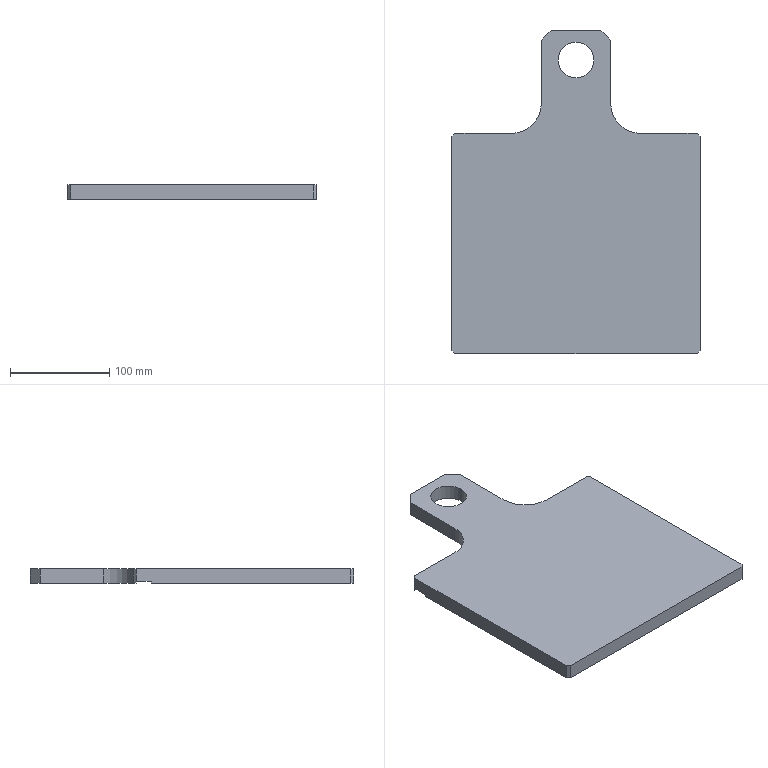Part | STEP file | 001-003-Shaft storage magazine support plate | 1 solid | 24 faces | box 250 x 326 x 15 mm | volume 922956 mm3 | plane 20 | cylinder 4 | commonest cylinder face diameters 36 x2 60 x2